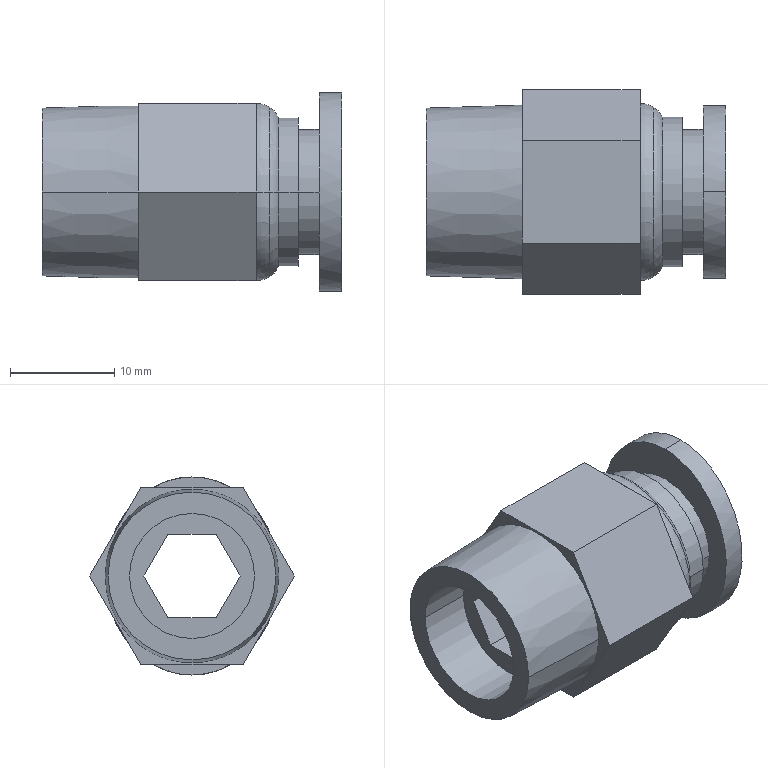Part | Creo | 1 solid | 45 faces | box 28.7 x 19.63 x 19 mm | volume 3914 mm3 | plane 25 | cylinder 8 | torus 8 | cone 2 | other 2 | commonest cylinder face diameters 12 x4 10 x2 14.36 x2
STEP:
#1=CARTESIAN_POINT('',(309.,102.978,120.));
#2=VERTEX_POINT('',#1);
#3=CARTESIAN_POINT('',(309.,114.978,120.));
#4=VERTEX_POINT('',#3);
#5=CARTESIAN_POINT('',(309.,108.978,120.));
#6=DIRECTION('',(-1.,0.,0.));
#7=DIRECTION('',(0.,-1.,0.));
#8=AXIS2_PLACEMENT_3D('',#5,#6,#7);
#9=CIRCLE('',#8,6.);
#10=EDGE_CURVE('',#2,#4,#9,.T.);
#11=ORIENTED_EDGE('',*,*,#10,.F.);
#12=CARTESIAN_POINT('',(309.,108.978,120.));
#13=DIRECTION('',(-1.,0.,0.));
#14=DIRECTION('',(0.,1.,0.));
#15=AXIS2_PLACEMENT_3D('',#12,#13,#14);
#16=CIRCLE('',#15,6.);
#17=EDGE_CURVE('',#4,#2,#16,.T.);
#18=ORIENTED_EDGE('',*,*,#17,.F.);
#19=EDGE_LOOP('',(#11,#18));
#20=FACE_OUTER_BOUND('',#19,.F.);
#21=CARTESIAN_POINT('',(309.,111.287,116.));
#22=VERTEX_POINT('',#21);
#23=CARTESIAN_POINT('',(309.,113.597,120.));
#24=VERTEX_POINT('',#23);
#25=CARTESIAN_POINT('',(309.,111.287,116.));
#26=DIRECTION('',(0.,0.5,0.866));
#27=VECTOR('',#26,4.619);
#28=LINE('',#25,#27);
#29=EDGE_CURVE('',#22,#24,#28,.T.);
#30=ORIENTED_EDGE('',*,*,#29,.F.);
#31=CARTESIAN_POINT('',(309.,106.668,116.));
#32=VERTEX_POINT('',#31);
#33=CARTESIAN_POINT('',(309.,106.668,116.));
#34=DIRECTION('',(0.,1.,0.));
#35=VECTOR('',#34,4.619);
#36=LINE('',#33,#35);
#37=EDGE_CURVE('',#32,#22,#36,.T.);
#38=ORIENTED_EDGE('',*,*,#37,.F.);
#39=CARTESIAN_POINT('',(309.,104.359,120.));
#40=VERTEX_POINT('',#39);
#41=CARTESIAN_POINT('',(309.,104.359,120.));
#42=DIRECTION('',(0.,0.5,-0.866));
#43=VECTOR('',#42,4.619);
#44=LINE('',#41,#43);
#45=EDGE_CURVE('',#40,#32,#44,.T.);
#46=ORIENTED_EDGE('',*,*,#45,.F.);
#47=CARTESIAN_POINT('',(309.,106.668,124.));
#48=VERTEX_POINT('',#47);
#49=CARTESIAN_POINT('',(309.,106.668,124.));
#50=DIRECTION('',(0.,-0.5,-0.866));
#51=VECTOR('',#50,4.619);
#52=LINE('',#49,#51);
#53=EDGE_CURVE('',#48,#40,#52,.T.);
#54=ORIENTED_EDGE('',*,*,#53,.F.);
#55=CARTESIAN_POINT('',(309.,111.287,124.));
#56=VERTEX_POINT('',#55);
#57=CARTESIAN_POINT('',(309.,111.287,124.));
#58=DIRECTION('',(0.,-1.,0.));
#59=VECTOR('',#58,4.619);
#60=LINE('',#57,#59);
#61=EDGE_CURVE('',#56,#48,#60,.T.);
#62=ORIENTED_EDGE('',*,*,#61,.F.);
#63=CARTESIAN_POINT('',(309.,113.597,120.));
#64=DIRECTION('',(0.,-0.5,0.866));
#65=VECTOR('',#64,4.619);
#66=LINE('',#63,#65);
#67=EDGE_CURVE('',#24,#56,#66,.T.);
#68=ORIENTED_EDGE('',*,*,#67,.F.);
#69=EDGE_LOOP('',(#30,#38,#46,#54,#62,#68));
#70=FACE_BOUND('',#69,.F.);
#71=CARTESIAN_POINT('',(309.,108.978,126.));
#72=DIRECTION('',(1.,0.,0.));
#73=DIRECTION('',(0.,1.,0.));
#74=AXIS2_PLACEMENT_3D('',#71,#72,#73);
#75=PLANE('',#74);
#76=ADVANCED_FACE('',(#20,#70),#75,.F.);
#77=CARTESIAN_POINT('',(303.8,114.978,120.));
#78=VERTEX_POINT('',#77);
#79=CARTESIAN_POINT('',(303.8,102.978,120.));
#80=VERTEX_POINT('',#79);
#81=CARTESIAN_POINT('',(303.8,108.978,120.));
#82=DIRECTION('',(1.,0.,0.));
#83=DIRECTION('',(0.,1.,0.));
#84=AXIS2_PLACEMENT_3D('',#81,#82,#83);
#85=CIRCLE('',#84,6.);
#86=EDGE_CURVE('',#78,#80,#85,.T.);
#87=ORIENTED_EDGE('',*,*,#86,.T.);
#88=CARTESIAN_POINT('',(309.,102.978,120.));
#89=DIRECTION('',(-1.,0.,0.));
#90=VECTOR('',#89,5.2);
#91=LINE('',#88,#90);
#92=EDGE_CURVE('',#2,#80,#91,.T.);
#93=ORIENTED_EDGE('',*,*,#92,.F.);
#94=ORIENTED_EDGE('',*,*,#10,.T.);
#95=CARTESIAN_POINT('',(309.,114.978,120.));
#96=DIRECTION('',(-1.,0.,0.));
#97=VECTOR('',#96,5.2);
#98=LINE('',#95,#97);
#99=EDGE_CURVE('',#4,#78,#98,.T.);
#100=ORIENTED_EDGE('',*,*,#99,.T.);
#101=EDGE_LOOP('',(#87,#93,#94,#100));
#102=FACE_OUTER_BOUND('',#101,.F.);
#103=CARTESIAN_POINT('',(335.,108.978,120.));
#104=DIRECTION('',(-1.,0.,0.));
#105=DIRECTION('',(0.,-1.,0.));
#106=AXIS2_PLACEMENT_3D('',#103,#104,#105);
#107=CYLINDRICAL_SURFACE('',#106,6.);
#108=ADVANCED_FACE('',(#102),#107,.F.);
#109=CARTESIAN_POINT('',(303.8,117.023,120.));
#110=VERTEX_POINT('',#109);
#111=CARTESIAN_POINT('',(303.8,100.933,120.));
#112=VERTEX_POINT('',#111);
#113=CARTESIAN_POINT('',(303.8,108.978,120.));
#114=DIRECTION('',(-1.,0.,0.));
#115=DIRECTION('',(0.,1.,0.));
#116=AXIS2_PLACEMENT_3D('',#113,#114,#115);
#117=CIRCLE('',#116,8.045);
#118=EDGE_CURVE('',#110,#112,#117,.T.);
#119=ORIENTED_EDGE('',*,*,#118,.F.);
#120=CARTESIAN_POINT('',(303.8,108.978,120.));
#121=DIRECTION('',(-1.,0.,0.));
#122=DIRECTION('',(0.,-1.,0.));
#123=AXIS2_PLACEMENT_3D('',#120,#121,#122);
#124=CIRCLE('',#123,8.045);
#125=EDGE_CURVE('',#112,#110,#124,.T.);
#126=ORIENTED_EDGE('',*,*,#125,.F.);
#127=EDGE_LOOP('',(#119,#126));
#128=FACE_OUTER_BOUND('',#127,.F.);
#129=CARTESIAN_POINT('',(303.8,108.978,120.));
#130=DIRECTION('',(1.,0.,0.));
#131=DIRECTION('',(0.,-1.,0.));
#132=AXIS2_PLACEMENT_3D('',#129,#130,#131);
#133=CIRCLE('',#132,6.);
#134=EDGE_CURVE('',#80,#78,#133,.T.);
#135=ORIENTED_EDGE('',*,*,#134,.F.);
#136=ORIENTED_EDGE('',*,*,#86,.F.);
#137=EDGE_LOOP('',(#135,#136));
#138=FACE_BOUND('',#137,.F.);
#139=CARTESIAN_POINT('',(303.8,108.978,128.045));
#140=DIRECTION('',(-1.,0.,0.));
#141=DIRECTION('',(0.,-1.,0.));
#142=AXIS2_PLACEMENT_3D('',#139,#140,#141);
#143=PLANE('',#142);
#144=ADVANCED_FACE('',(#128,#138),#143,.T.);
#145=ORIENTED_EDGE('',*,*,#134,.T.);
#146=ORIENTED_EDGE('',*,*,#99,.F.);
#147=ORIENTED_EDGE('',*,*,#17,.T.);
#148=ORIENTED_EDGE('',*,*,#92,.T.);
#149=EDGE_LOOP('',(#145,#146,#147,#148));
#150=FACE_OUTER_BOUND('',#149,.F.);
#151=CARTESIAN_POINT('',(335.,108.978,120.));
#152=DIRECTION('',(-1.,0.,0.));
#153=DIRECTION('',(0.,-1.,0.));
#154=AXIS2_PLACEMENT_3D('',#151,#152,#153);
#155=CYLINDRICAL_SURFACE('',#154,6.);
#156=ADVANCED_FACE('',(#150),#155,.F.);
#157=ORIENTED_EDGE('',*,*,#118,.T.);
#158=CARTESIAN_POINT('',(313.,100.648,120.));
#159=VERTEX_POINT('',#158);
#160=CARTESIAN_POINT('',(303.8,100.933,120.));
#161=DIRECTION('',(0.9995,-0.03097,0.));
#162=VECTOR('',#161,9.204);
#163=LINE('',#160,#162);
#164=EDGE_CURVE('',#112,#159,#163,.T.);
#165=ORIENTED_EDGE('',*,*,#164,.T.);
#166=CARTESIAN_POINT('',(313.,117.308,120.));
#167=VERTEX_POINT('',#166);
#168=CARTESIAN_POINT('',(313.,108.978,120.));
#169=DIRECTION('',(1.,0.,0.));
#170=DIRECTION('',(0.,-1.,0.));
#171=AXIS2_PLACEMENT_3D('',#168,#169,#170);
#172=CIRCLE('',#171,8.33);
#173=EDGE_CURVE('',#159,#167,#172,.T.);
#174=ORIENTED_EDGE('',*,*,#173,.T.);
#175=CARTESIAN_POINT('',(303.8,117.023,120.));
#176=DIRECTION('',(0.9995,0.03097,0.));
#177=VECTOR('',#176,9.204);
#178=LINE('',#175,#177);
#179=EDGE_CURVE('',#110,#167,#178,.T.);
#180=ORIENTED_EDGE('',*,*,#179,.F.);
#181=EDGE_LOOP('',(#157,#165,#174,#180));
#182=FACE_OUTER_BOUND('',#181,.F.);
#183=CARTESIAN_POINT('',(308.4,108.978,120.));
#184=DIRECTION('',(1.,0.,0.));
#185=DIRECTION('',(0.,1.,0.));
#186=AXIS2_PLACEMENT_3D('',#183,#184,#185);
#187=CONICAL_SURFACE('',#186,8.187,1.775);
#188=ADVANCED_FACE('',(#182),#187,.T.);
#189=ORIENTED_EDGE('',*,*,#125,.T.);
#190=ORIENTED_EDGE('',*,*,#179,.T.);
#191=CARTESIAN_POINT('',(313.,108.978,120.));
#192=DIRECTION('',(1.,0.,0.));
#193=DIRECTION('',(0.,1.,0.));
#194=AXIS2_PLACEMENT_3D('',#191,#192,#193);
#195=CIRCLE('',#194,8.33);
#196=EDGE_CURVE('',#167,#159,#195,.T.);
#197=ORIENTED_EDGE('',*,*,#196,.T.);
#198=ORIENTED_EDGE('',*,*,#164,.F.);
#199=EDGE_LOOP('',(#189,#190,#197,#198));
#200=FACE_OUTER_BOUND('',#199,.F.);
#201=CARTESIAN_POINT('',(308.4,108.978,120.));
#202=DIRECTION('',(1.,0.,0.));
#203=DIRECTION('',(0.,1.,0.));
#204=AXIS2_PLACEMENT_3D('',#201,#202,#203);
#205=CONICAL_SURFACE('',#204,8.187,1.775);
#206=ADVANCED_FACE('',(#200),#205,.T.);
#207=CARTESIAN_POINT('',(313.,99.163,120.));
#208=VERTEX_POINT('',#207);
#209=CARTESIAN_POINT('',(313.,104.07,128.5));
#210=VERTEX_POINT('',#209);
#211=CARTESIAN_POINT('',(313.,99.163,120.));
#212=DIRECTION('',(0.,0.5,0.866));
#213=VECTOR('',#212,9.815);
#214=LINE('',#211,#213);
#215=EDGE_CURVE('',#208,#210,#214,.T.);
#216=ORIENTED_EDGE('',*,*,#215,.F.);
#217=CARTESIAN_POINT('',(313.,104.07,111.5));
#218=VERTEX_POINT('',#217);
#219=CARTESIAN_POINT('',(313.,104.07,111.5));
#220=DIRECTION('',(0.,-0.5,0.866));
#221=VECTOR('',#220,9.815);
#222=LINE('',#219,#221);
#223=EDGE_CURVE('',#218,#208,#222,.T.);
#224=ORIENTED_EDGE('',*,*,#223,.F.);
#225=CARTESIAN_POINT('',(313.,113.885,111.5));
#226=VERTEX_POINT('',#225);
#227=CARTESIAN_POINT('',(313.,104.07,111.5));
#228=DIRECTION('',(0.,1.,0.));
#229=VECTOR('',#228,9.815);
#230=LINE('',#227,#229);
#231=EDGE_CURVE('',#218,#226,#230,.T.);
#232=ORIENTED_EDGE('',*,*,#231,.T.);
#233=CARTESIAN_POINT('',(313.,118.793,120.));
#234=VERTEX_POINT('',#233);
#235=CARTESIAN_POINT('',(313.,118.793,120.));
#236=DIRECTION('',(0.,-0.5,-0.866));
#237=VECTOR('',#236,9.815);
#238=LINE('',#235,#237);
#239=EDGE_CURVE('',#234,#226,#238,.T.);
#240=ORIENTED_EDGE('',*,*,#239,.F.);
#241=CARTESIAN_POINT('',(313.,113.885,128.5));
#242=VERTEX_POINT('',#241);
#243=CARTESIAN_POINT('',(313.,113.885,128.5));
#244=DIRECTION('',(0.,0.5,-0.866));
#245=VECTOR('',#244,9.815);
#246=LINE('',#243,#245);
#247=EDGE_CURVE('',#242,#234,#246,.T.);
#248=ORIENTED_EDGE('',*,*,#247,.F.);
#249=CARTESIAN_POINT('',(313.,113.885,128.5));
#250=DIRECTION('',(0.,-1.,0.));
#251=VECTOR('',#250,9.815);
#252=LINE('',#249,#251);
#253=EDGE_CURVE('',#242,#210,#252,.T.);
#254=ORIENTED_EDGE('',*,*,#253,.T.);
#255=EDGE_LOOP('',(#216,#224,#232,#240,#248,#254));
#256=FACE_OUTER_BOUND('',#255,.F.);
#257=ORIENTED_EDGE('',*,*,#196,.F.);
#258=ORIENTED_EDGE('',*,*,#173,.F.);
#259=EDGE_LOOP('',(#257,#258));
#260=FACE_BOUND('',#259,.F.);
#261=CARTESIAN_POINT('',(313.,108.978,128.4));
#262=DIRECTION('',(-1.,0.,0.));
#263=DIRECTION('',(0.,-1.,0.));
#264=AXIS2_PLACEMENT_3D('',#261,#262,#263);
#265=PLANE('',#264);
#266=ADVANCED_FACE('',(#256,#260),#265,.T.);
#267=ORIENTED_EDGE('',*,*,#215,.T.);
#268=CARTESIAN_POINT('',(324.3,104.07,128.5));
#269=VERTEX_POINT('',#268);
#270=CARTESIAN_POINT('',(313.,104.07,128.5));
#271=DIRECTION('',(1.,0.,0.));
#272=VECTOR('',#271,11.3);
#273=LINE('',#270,#272);
#274=EDGE_CURVE('',#210,#269,#273,.T.);
#275=ORIENTED_EDGE('',*,*,#274,.T.);
#276=CARTESIAN_POINT('',(324.3,101.617,124.25));
#277=VERTEX_POINT('',#276);
#278=CARTESIAN_POINT('',(324.3,104.07,128.5));
#279=DIRECTION('',(0.,-0.5,-0.866));
#280=VECTOR('',#279,4.907);
#281=LINE('',#278,#280);
#282=EDGE_CURVE('',#269,#277,#281,.T.);
#283=ORIENTED_EDGE('',*,*,#282,.T.);
#284=CARTESIAN_POINT('',(324.3,99.163,120.));
#285=VERTEX_POINT('',#284);
#286=CARTESIAN_POINT('',(324.3,101.617,124.25));
#287=DIRECTION('',(0.,-0.5,-0.866));
#288=VECTOR('',#287,4.907);
#289=LINE('',#286,#288);
#290=EDGE_CURVE('',#277,#285,#289,.T.);
#291=ORIENTED_EDGE('',*,*,#290,.T.);
#292=CARTESIAN_POINT('',(313.,99.163,120.));
#293=DIRECTION('',(1.,0.,0.));
#294=VECTOR('',#293,11.3);
#295=LINE('',#292,#294);
#296=EDGE_CURVE('',#208,#285,#295,.T.);
#297=ORIENTED_EDGE('',*,*,#296,.F.);
#298=EDGE_LOOP('',(#267,#275,#283,#291,#297));
#299=FACE_OUTER_BOUND('',#298,.F.);
#300=CARTESIAN_POINT('',(324.3,99.163,120.));
#301=DIRECTION('',(0.,-0.866,0.5));
#302=DIRECTION('',(0.,-0.5,-0.866));
#303=AXIS2_PLACEMENT_3D('',#300,#301,#302);
#304=PLANE('',#303);
#305=ADVANCED_FACE('',(#299),#304,.T.);
#306=ORIENTED_EDGE('',*,*,#253,.F.);
#307=CARTESIAN_POINT('',(324.3,113.885,128.5));
#308=VERTEX_POINT('',#307);
#309=CARTESIAN_POINT('',(313.,113.885,128.5));
#310=DIRECTION('',(1.,0.,0.));
#311=VECTOR('',#310,11.3);
#312=LINE('',#309,#311);
#313=EDGE_CURVE('',#242,#308,#312,.T.);
#314=ORIENTED_EDGE('',*,*,#313,.T.);
#315=CARTESIAN_POINT('',(324.3,108.978,128.5));
#316=VERTEX_POINT('',#315);
#317=CARTESIAN_POINT('',(324.3,113.885,128.5));
#318=DIRECTION('',(0.,-1.,0.));
#319=VECTOR('',#318,4.907);
#320=LINE('',#317,#319);
#321=EDGE_CURVE('',#308,#316,#320,.T.);
#322=ORIENTED_EDGE('',*,*,#321,.T.);
#323=CARTESIAN_POINT('',(324.3,108.978,128.5));
#324=DIRECTION('',(0.,-1.,0.));
#325=VECTOR('',#324,4.907);
#326=LINE('',#323,#325);
#327=EDGE_CURVE('',#316,#269,#326,.T.);
#328=ORIENTED_EDGE('',*,*,#327,.T.);
#329=ORIENTED_EDGE('',*,*,#274,.F.);
#330=EDGE_LOOP('',(#306,#314,#322,#328,#329));
#331=FACE_OUTER_BOUND('',#330,.F.);
#332=CARTESIAN_POINT('',(324.3,104.07,128.5));
#333=DIRECTION('',(0.,0.,1.));
#334=DIRECTION('',(1.,0.,0.));
#335=AXIS2_PLACEMENT_3D('',#332,#333,#334);
#336=PLANE('',#335);
#337=ADVANCED_FACE('',(#331),#336,.T.);
#338=CARTESIAN_POINT('',(324.3,118.793,120.));
#339=VERTEX_POINT('',#338);
#340=CARTESIAN_POINT('',(313.,118.793,120.));
#341=DIRECTION('',(1.,0.,0.));
#342=VECTOR('',#341,11.3);
#343=LINE('',#340,#342);
#344=EDGE_CURVE('',#234,#339,#343,.T.);
#345=ORIENTED_EDGE('',*,*,#344,.T.);
#346=CARTESIAN_POINT('',(324.3,116.339,124.25));
#347=VERTEX_POINT('',#346);
#348=CARTESIAN_POINT('',(324.3,118.793,120.));
#349=DIRECTION('',(0.,-0.5,0.866));
#350=VECTOR('',#349,4.907);
#351=LINE('',#348,#350);
#352=EDGE_CURVE('',#339,#347,#351,.T.);
#353=ORIENTED_EDGE('',*,*,#352,.T.);
#354=CARTESIAN_POINT('',(324.3,116.339,124.25));
#355=DIRECTION('',(0.,-0.5,0.866));
#356=VECTOR('',#355,4.907);
#357=LINE('',#354,#356);
#358=EDGE_CURVE('',#347,#308,#357,.T.);
#359=ORIENTED_EDGE('',*,*,#358,.T.);
#360=ORIENTED_EDGE('',*,*,#313,.F.);
#361=ORIENTED_EDGE('',*,*,#247,.T.);
#362=EDGE_LOOP('',(#345,#353,#359,#360,#361));
#363=FACE_OUTER_BOUND('',#362,.F.);
#364=CARTESIAN_POINT('',(324.3,113.885,128.5));
#365=DIRECTION('',(0.,0.866,0.5));
#366=DIRECTION('',(0.,-0.5,0.866));
#367=AXIS2_PLACEMENT_3D('',#364,#365,#366);
#368=PLANE('',#367);
#369=ADVANCED_FACE('',(#363),#368,.T.);
#370=ORIENTED_EDGE('',*,*,#239,.T.);
#371=CARTESIAN_POINT('',(324.3,113.885,111.5));
#372=VERTEX_POINT('',#371);
#373=CARTESIAN_POINT('',(313.,113.885,111.5));
#374=DIRECTION('',(1.,0.,0.));
#375=VECTOR('',#374,11.3);
#376=LINE('',#373,#375);
#377=EDGE_CURVE('',#226,#372,#376,.T.);
#378=ORIENTED_EDGE('',*,*,#377,.T.);
#379=CARTESIAN_POINT('',(324.3,116.339,115.75));
#380=VERTEX_POINT('',#379);
#381=CARTESIAN_POINT('',(324.3,113.885,111.5));
#382=DIRECTION('',(0.,0.5,0.866));
#383=VECTOR('',#382,4.907);
#384=LINE('',#381,#383);
#385=EDGE_CURVE('',#372,#380,#384,.T.);
#386=ORIENTED_EDGE('',*,*,#385,.T.);
#387=CARTESIAN_POINT('',(324.3,116.339,115.75));
#388=DIRECTION('',(0.,0.5,0.866));
#389=VECTOR('',#388,4.907);
#390=LINE('',#387,#389);
#391=EDGE_CURVE('',#380,#339,#390,.T.);
#392=ORIENTED_EDGE('',*,*,#391,.T.);
#393=ORIENTED_EDGE('',*,*,#344,.F.);
#394=EDGE_LOOP('',(#370,#378,#386,#392,#393));
#395=FACE_OUTER_BOUND('',#394,.F.);
#396=CARTESIAN_POINT('',(324.3,118.793,120.));
#397=DIRECTION('',(0.,0.866,-0.5));
#398=DIRECTION('',(0.,0.5,0.866));
#399=AXIS2_PLACEMENT_3D('',#396,#397,#398);
#400=PLANE('',#399);
#401=ADVANCED_FACE('',(#395),#400,.T.);
#402=ORIENTED_EDGE('',*,*,#231,.F.);
#403=CARTESIAN_POINT('',(324.3,104.07,111.5));
#404=VERTEX_POINT('',#403);
#405=CARTESIAN_POINT('',(313.,104.07,111.5));
#406=DIRECTION('',(1.,0.,0.));
#407=VECTOR('',#406,11.3);
#408=LINE('',#405,#407);
#409=EDGE_CURVE('',#218,#404,#408,.T.);
#410=ORIENTED_EDGE('',*,*,#409,.T.);
#411=CARTESIAN_POINT('',(324.3,108.978,111.5));
#412=VERTEX_POINT('',#411);
#413=CARTESIAN_POINT('',(324.3,104.07,111.5));
#414=DIRECTION('',(0.,1.,0.));
#415=VECTOR('',#414,4.907);
#416=LINE('',#413,#415);
#417=EDGE_CURVE('',#404,#412,#416,.T.);
#418=ORIENTED_EDGE('',*,*,#417,.T.);
#419=CARTESIAN_POINT('',(324.3,108.978,111.5));
#420=DIRECTION('',(0.,1.,0.));
#421=VECTOR('',#420,4.907);
#422=LINE('',#419,#421);
#423=EDGE_CURVE('',#412,#372,#422,.T.);
#424=ORIENTED_EDGE('',*,*,#423,.T.);
#425=ORIENTED_EDGE('',*,*,#377,.F.);
#426=EDGE_LOOP('',(#402,#410,#418,#424,#425));
#427=FACE_OUTER_BOUND('',#426,.F.);
#428=CARTESIAN_POINT('',(324.3,113.885,111.5));
#429=DIRECTION('',(0.,0.,-1.));
#430=DIRECTION('',(0.,1.,0.));
#431=AXIS2_PLACEMENT_3D('',#428,#429,#430);
#432=PLANE('',#431);
#433=ADVANCED_FACE('',(#427),#432,.T.);
#434=ORIENTED_EDGE('',*,*,#223,.T.);
#435=ORIENTED_EDGE('',*,*,#296,.T.);
#436=CARTESIAN_POINT('',(324.3,101.617,115.75));
#437=VERTEX_POINT('',#436);
#438=CARTESIAN_POINT('',(324.3,99.163,120.));
#439=DIRECTION('',(0.,0.5,-0.866));
#440=VECTOR('',#439,4.907);
#441=LINE('',#438,#440);
#442=EDGE_CURVE('',#285,#437,#441,.T.);
#443=ORIENTED_EDGE('',*,*,#442,.T.);
#444=CARTESIAN_POINT('',(324.3,101.617,115.75));
#445=DIRECTION('',(0.,0.5,-0.866));
#446=VECTOR('',#445,4.907);
#447=LINE('',#444,#446);
#448=EDGE_CURVE('',#437,#404,#447,.T.);
#449=ORIENTED_EDGE('',*,*,#448,.T.);
#450=ORIENTED_EDGE('',*,*,#409,.F.);
#451=EDGE_LOOP('',(#434,#435,#443,#449,#450));
#452=FACE_OUTER_BOUND('',#451,.F.);
#453=CARTESIAN_POINT('',(324.3,104.07,111.5));
#454=DIRECTION('',(0.,-0.866,-0.5));
#455=DIRECTION('',(0.,0.5,-0.866));
#456=AXIS2_PLACEMENT_3D('',#453,#454,#455);
#457=PLANE('',#456);
#458=ADVANCED_FACE('',(#452),#457,.T.);
#459=CARTESIAN_POINT('',(324.3,100.478,120.));
#460=VERTEX_POINT('',#459);
#461=CARTESIAN_POINT('',(324.3,108.978,120.));
#462=DIRECTION('',(-1.,0.,0.));
#463=DIRECTION('',(0.,-0.866,-0.5));
#464=AXIS2_PLACEMENT_3D('',#461,#462,#463);
#465=CIRCLE('',#464,8.5);
#466=EDGE_CURVE('',#437,#460,#465,.T.);
#467=ORIENTED_EDGE('',*,*,#466,.F.);
#468=ORIENTED_EDGE('',*,*,#442,.F.);
#469=ORIENTED_EDGE('',*,*,#290,.F.);
#470=CARTESIAN_POINT('',(324.3,108.978,120.));
#471=DIRECTION('',(-1.,0.,0.));
#472=DIRECTION('',(0.,-1.,0.));
#473=AXIS2_PLACEMENT_3D('',#470,#471,#472);
#474=CIRCLE('',#473,8.5);
#475=EDGE_CURVE('',#460,#277,#474,.T.);
#476=ORIENTED_EDGE('',*,*,#475,.F.);
#477=EDGE_LOOP('',(#467,#468,#469,#476));
#478=FACE_OUTER_BOUND('',#477,.F.);
#479=CARTESIAN_POINT('',(324.3,108.978,120.));
#480=DIRECTION('',(-1.,0.,0.));
#481=DIRECTION('',(0.,-1.,0.));
#482=AXIS2_PLACEMENT_3D('',#479,#480,#481);
#483=PLANE('',#482);
#484=ADVANCED_FACE('',(#478),#483,.F.);
#485=ORIENTED_EDGE('',*,*,#466,.T.);
#486=CARTESIAN_POINT('',(325.561,100.834,120.));
#487=VERTEX_POINT('',#486);
#488=CARTESIAN_POINT('',(324.3,102.889,120.));
#489=DIRECTION('',(0.,0.,1.));
#490=DIRECTION('',(0.,-1.,0.));
#491=AXIS2_PLACEMENT_3D('',#488,#489,#490);
#492=CIRCLE('',#491,2.411);
#493=EDGE_CURVE('',#460,#487,#492,.T.);
#494=ORIENTED_EDGE('',*,*,#493,.T.);
#495=CARTESIAN_POINT('',(325.561,117.121,120.));
#496=VERTEX_POINT('',#495);
#497=CARTESIAN_POINT('',(325.561,108.978,120.));
#498=DIRECTION('',(1.,0.,0.));
#499=DIRECTION('',(0.,-1.,0.));
#500=AXIS2_PLACEMENT_3D('',#497,#498,#499);
#501=CIRCLE('',#500,8.144);
#502=EDGE_CURVE('',#487,#496,#501,.T.);
#503=ORIENTED_EDGE('',*,*,#502,.T.);
#504=CARTESIAN_POINT('',(324.3,117.478,120.));
#505=VERTEX_POINT('',#504);
#506=CARTESIAN_POINT('',(324.3,115.067,120.));
#507=DIRECTION('',(0.,0.,-1.));
#508=DIRECTION('',(0.,1.,0.));
#509=AXIS2_PLACEMENT_3D('',#506,#507,#508);
#510=CIRCLE('',#509,2.411);
#511=EDGE_CURVE('',#505,#496,#510,.T.);
#512=ORIENTED_EDGE('',*,*,#511,.F.);
#513=CARTESIAN_POINT('',(324.3,108.978,120.));
#514=DIRECTION('',(-1.,0.,0.));
#515=DIRECTION('',(0.,1.,0.));
#516=AXIS2_PLACEMENT_3D('',#513,#514,#515);
#517=CIRCLE('',#516,8.5);
#518=EDGE_CURVE('',#505,#380,#517,.T.);
#519=ORIENTED_EDGE('',*,*,#518,.T.);
#520=CARTESIAN_POINT('',(324.3,108.978,120.));
#521=DIRECTION('',(-1.,0.,0.));
#522=DIRECTION('',(0.,0.866,-0.5));
#523=AXIS2_PLACEMENT_3D('',#520,#521,#522);
#524=CIRCLE('',#523,8.5);
#525=EDGE_CURVE('',#380,#412,#524,.T.);
#526=ORIENTED_EDGE('',*,*,#525,.T.);
#527=CARTESIAN_POINT('',(324.3,108.978,120.));
#528=DIRECTION('',(-1.,0.,0.));
#529=DIRECTION('',(0.,0.,-1.));
#530=AXIS2_PLACEMENT_3D('',#527,#528,#529);
#531=CIRCLE('',#530,8.5);
#532=EDGE_CURVE('',#412,#437,#531,.T.);
#533=ORIENTED_EDGE('',*,*,#532,.T.);
#534=EDGE_LOOP('',(#485,#494,#503,#512,#519,#526,#533));
#535=FACE_OUTER_BOUND('',#534,.F.);
#536=CARTESIAN_POINT('',(324.3,108.978,120.));
#537=DIRECTION('',(1.,0.,0.));
#538=DIRECTION('',(0.,1.,0.));
#539=AXIS2_PLACEMENT_3D('',#536,#537,#538);
#540=TOROIDAL_SURFACE('',#539,6.089,2.411);
#541=ADVANCED_FACE('',(#535),#540,.T.);
#542=CARTESIAN_POINT('',(324.3,108.978,120.));
#543=DIRECTION('',(-1.,0.,0.));
#544=DIRECTION('',(0.,0.,1.));
#545=AXIS2_PLACEMENT_3D('',#542,#543,#544);
#546=CIRCLE('',#545,8.5);
#547=EDGE_CURVE('',#316,#347,#546,.T.);
#548=ORIENTED_EDGE('',*,*,#547,.T.);
#549=CARTESIAN_POINT('',(324.3,108.978,120.));
#550=DIRECTION('',(-1.,0.,0.));
#551=DIRECTION('',(0.,0.866,0.5));
#552=AXIS2_PLACEMENT_3D('',#549,#550,#551);
#553=CIRCLE('',#552,8.5);
#554=EDGE_CURVE('',#347,#505,#553,.T.);
#555=ORIENTED_EDGE('',*,*,#554,.T.);
#556=ORIENTED_EDGE('',*,*,#511,.T.);
#557=CARTESIAN_POINT('',(325.561,108.978,120.));
#558=DIRECTION('',(1.,0.,0.));
#559=DIRECTION('',(0.,1.,0.));
#560=AXIS2_PLACEMENT_3D('',#557,#558,#559);
#561=CIRCLE('',#560,8.144);
#562=EDGE_CURVE('',#496,#487,#561,.T.);
#563=ORIENTED_EDGE('',*,*,#562,.T.);
#564=ORIENTED_EDGE('',*,*,#493,.F.);
#565=ORIENTED_EDGE('',*,*,#475,.T.);
#566=CARTESIAN_POINT('',(324.3,108.978,120.));
#567=DIRECTION('',(-1.,0.,0.));
#568=DIRECTION('',(0.,-0.866,0.5));
#569=AXIS2_PLACEMENT_3D('',#566,#567,#568);
#570=CIRCLE('',#569,8.5);
#571=EDGE_CURVE('',#277,#316,#570,.T.);
#572=ORIENTED_EDGE('',*,*,#571,.T.);
#573=EDGE_LOOP('',(#548,#555,#556,#563,#564,#565,#572));
#574=FACE_OUTER_BOUND('',#573,.F.);
#575=CARTESIAN_POINT('',(324.3,108.978,120.));
#576=DIRECTION('',(1.,0.,0.));
#577=DIRECTION('',(0.,1.,0.));
#578=AXIS2_PLACEMENT_3D('',#575,#576,#577);
#579=TOROIDAL_SURFACE('',#578,6.089,2.411);
#580=ADVANCED_FACE('',(#574),#579,.T.);
#581=ORIENTED_EDGE('',*,*,#547,.F.);
#582=ORIENTED_EDGE('',*,*,#321,.F.);
#583=ORIENTED_EDGE('',*,*,#358,.F.);
#584=EDGE_LOOP('',(#581,#582,#583));
#585=FACE_OUTER_BOUND('',#584,.F.);
#586=CARTESIAN_POINT('',(324.3,108.978,120.));
#587=DIRECTION('',(-1.,0.,0.));
#588=DIRECTION('',(0.,-1.,0.));
#589=AXIS2_PLACEMENT_3D('',#586,#587,#588);
#590=PLANE('',#589);
#591=ADVANCED_FACE('',(#585),#590,.F.);
#592=ORIENTED_EDGE('',*,*,#518,.F.);
#593=ORIENTED_EDGE('',*,*,#554,.F.);
#594=ORIENTED_EDGE('',*,*,#352,.F.);
#595=ORIENTED_EDGE('',*,*,#391,.F.);
#596=EDGE_LOOP('',(#592,#593,#594,#595));
#597=FACE_OUTER_BOUND('',#596,.F.);
#598=CARTESIAN_POINT('',(324.3,108.978,120.));
#599=DIRECTION('',(-1.,0.,0.));
#600=DIRECTION('',(0.,-1.,0.));
#601=AXIS2_PLACEMENT_3D('',#598,#599,#600);
#602=PLANE('',#601);
#603=ADVANCED_FACE('',(#597),#602,.F.);
#604=CARTESIAN_POINT('',(326.45,101.798,120.));
#605=VERTEX_POINT('',#604);
#606=CARTESIAN_POINT('',(326.45,116.158,120.));
#607=VERTEX_POINT('',#606);
#608=CARTESIAN_POINT('',(326.45,108.978,120.));
#609=DIRECTION('',(-1.,0.,0.));
#610=DIRECTION('',(0.,-1.,0.));
#611=AXIS2_PLACEMENT_3D('',#608,#609,#610);
#612=CIRCLE('',#611,7.18);
#613=EDGE_CURVE('',#605,#607,#612,.T.);
#614=ORIENTED_EDGE('',*,*,#613,.F.);
#615=CARTESIAN_POINT('',(324.3,102.889,120.));
#616=DIRECTION('',(0.,0.,1.));
#617=DIRECTION('',(0.5232,-0.8522,0.));
#618=AXIS2_PLACEMENT_3D('',#615,#616,#617);
#619=CIRCLE('',#618,2.411);
#620=EDGE_CURVE('',#487,#605,#619,.T.);
#621=ORIENTED_EDGE('',*,*,#620,.F.);
#622=ORIENTED_EDGE('',*,*,#562,.F.);
#623=CARTESIAN_POINT('',(324.3,115.067,120.));
#624=DIRECTION('',(0.,0.,-1.));
#625=DIRECTION('',(0.5232,0.8522,0.));
#626=AXIS2_PLACEMENT_3D('',#623,#624,#625);
#627=CIRCLE('',#626,2.411);
#628=EDGE_CURVE('',#496,#607,#627,.T.);
#629=ORIENTED_EDGE('',*,*,#628,.T.);
#630=EDGE_LOOP('',(#614,#621,#622,#629));
#631=FACE_OUTER_BOUND('',#630,.F.);
#632=CARTESIAN_POINT('',(324.3,108.978,120.));
#633=DIRECTION('',(1.,0.,0.));
#634=DIRECTION('',(0.,1.,0.));
#635=AXIS2_PLACEMENT_3D('',#632,#633,#634);
#636=TOROIDAL_SURFACE('',#635,6.089,2.411);
#637=ADVANCED_FACE('',(#631),#636,.T.);
#638=ORIENTED_EDGE('',*,*,#613,.T.);
#639=CARTESIAN_POINT('',(328.35,116.158,120.));
#640=VERTEX_POINT('',#639);
#641=CARTESIAN_POINT('',(326.45,116.158,120.));
#642=DIRECTION('',(1.,0.,0.));
#643=VECTOR('',#642,1.9);
#644=LINE('',#641,#643);
#645=EDGE_CURVE('',#607,#640,#644,.T.);
#646=ORIENTED_EDGE('',*,*,#645,.T.);
#647=CARTESIAN_POINT('',(328.35,101.798,120.));
#648=VERTEX_POINT('',#647);
#649=CARTESIAN_POINT('',(328.35,108.978,120.));
#650=DIRECTION('',(1.,0.,0.));
#651=DIRECTION('',(0.,1.,0.));
#652=AXIS2_PLACEMENT_3D('',#649,#650,#651);
#653=CIRCLE('',#652,7.18);
#654=EDGE_CURVE('',#640,#648,#653,.T.);
#655=ORIENTED_EDGE('',*,*,#654,.T.);
#656=CARTESIAN_POINT('',(326.45,101.798,120.));
#657=DIRECTION('',(1.,0.,0.));
#658=VECTOR('',#657,1.9);
#659=LINE('',#656,#658);
#660=EDGE_CURVE('',#605,#648,#659,.T.);
#661=ORIENTED_EDGE('',*,*,#660,.F.);
#662=EDGE_LOOP('',(#638,#646,#655,#661));
#663=FACE_OUTER_BOUND('',#662,.F.);
#664=CARTESIAN_POINT('',(335.,108.978,120.));
#665=DIRECTION('',(1.,0.,0.));
#666=DIRECTION('',(0.,1.,0.));
#667=AXIS2_PLACEMENT_3D('',#664,#665,#666);
#668=CYLINDRICAL_SURFACE('',#667,7.18);
#669=ADVANCED_FACE('',(#663),#668,.T.);
#670=CARTESIAN_POINT('',(326.45,108.978,120.));
#671=DIRECTION('',(-1.,0.,0.));
#672=DIRECTION('',(0.,1.,0.));
#673=AXIS2_PLACEMENT_3D('',#670,#671,#672);
#674=CIRCLE('',#673,7.18);
#675=EDGE_CURVE('',#607,#605,#674,.T.);
#676=ORIENTED_EDGE('',*,*,#675,.T.);
#677=ORIENTED_EDGE('',*,*,#660,.T.);
#678=CARTESIAN_POINT('',(328.35,108.978,120.));
#679=DIRECTION('',(1.,0.,0.));
#680=DIRECTION('',(0.,-1.,0.));
#681=AXIS2_PLACEMENT_3D('',#678,#679,#680);
#682=CIRCLE('',#681,7.18);
#683=EDGE_CURVE('',#648,#640,#682,.T.);
#684=ORIENTED_EDGE('',*,*,#683,.T.);
#685=ORIENTED_EDGE('',*,*,#645,.F.);
#686=EDGE_LOOP('',(#676,#677,#684,#685));
#687=FACE_OUTER_BOUND('',#686,.F.);
#688=CARTESIAN_POINT('',(335.,108.978,120.));
#689=DIRECTION('',(1.,0.,0.));
#690=DIRECTION('',(0.,1.,0.));
#691=AXIS2_PLACEMENT_3D('',#688,#689,#690);
#692=CYLINDRICAL_SURFACE('',#691,7.18);
#693=ADVANCED_FACE('',(#687),#692,.T.);
#694=ORIENTED_EDGE('',*,*,#675,.F.);
#695=ORIENTED_EDGE('',*,*,#628,.F.);
#696=ORIENTED_EDGE('',*,*,#502,.F.);
#697=ORIENTED_EDGE('',*,*,#620,.T.);
#698=EDGE_LOOP('',(#694,#695,#696,#697));
#699=FACE_OUTER_BOUND('',#698,.F.);
#700=CARTESIAN_POINT('',(324.3,108.978,120.));
#701=DIRECTION('',(1.,0.,0.));
#702=DIRECTION('',(0.,1.,0.));
#703=AXIS2_PLACEMENT_3D('',#700,#701,#702);
#704=TOROIDAL_SURFACE('',#703,6.089,2.411);
#705=ADVANCED_FACE('',(#699),#704,.T.);
#706=ORIENTED_EDGE('',*,*,#654,.F.);
#707=ORIENTED_EDGE('',*,*,#683,.F.);
#708=EDGE_LOOP('',(#706,#707));
#709=FACE_OUTER_BOUND('',#708,.F.);
#710=CARTESIAN_POINT('',(328.35,114.978,120.));
#711=VERTEX_POINT('',#710);
#712=CARTESIAN_POINT('',(328.35,102.978,120.));
#713=VERTEX_POINT('',#712);
#714=CARTESIAN_POINT('',(328.35,108.978,120.));
#715=DIRECTION('',(-1.,0.,0.));
#716=DIRECTION('',(0.,1.,0.));
#717=AXIS2_PLACEMENT_3D('',#714,#715,#716);
#718=CIRCLE('',#717,6.);
#719=EDGE_CURVE('',#711,#713,#718,.T.);
#720=ORIENTED_EDGE('',*,*,#719,.F.);
#721=CARTESIAN_POINT('',(328.35,108.978,120.));
#722=DIRECTION('',(-1.,0.,0.));
#723=DIRECTION('',(0.,-1.,0.));
#724=AXIS2_PLACEMENT_3D('',#721,#722,#723);
#725=CIRCLE('',#724,6.);
#726=EDGE_CURVE('',#713,#711,#725,.T.);
#727=ORIENTED_EDGE('',*,*,#726,.F.);
#728=EDGE_LOOP('',(#720,#727));
#729=FACE_BOUND('',#728,.F.);
#730=CARTESIAN_POINT('',(328.35,108.978,126.));
#731=DIRECTION('',(1.,0.,0.));
#732=DIRECTION('',(0.,1.,0.));
#733=AXIS2_PLACEMENT_3D('',#730,#731,#732);
#734=PLANE('',#733);
#735=ADVANCED_FACE('',(#709,#729),#734,.T.);
#736=ORIENTED_EDGE('',*,*,#719,.T.);
#737=CARTESIAN_POINT('',(330.35,102.978,120.));
#738=VERTEX_POINT('',#737);
#739=CARTESIAN_POINT('',(328.35,102.978,120.));
#740=DIRECTION('',(1.,0.,0.));
#741=VECTOR('',#740,2.);
#742=LINE('',#739,#741);
#743=EDGE_CURVE('',#713,#738,#742,.T.);
#744=ORIENTED_EDGE('',*,*,#743,.T.);
#745=CARTESIAN_POINT('',(330.35,114.978,120.));
#746=VERTEX_POINT('',#745);
#747=CARTESIAN_POINT('',(330.35,108.978,120.));
#748=DIRECTION('',(1.,0.,0.));
#749=DIRECTION('',(0.,-1.,0.));
#750=AXIS2_PLACEMENT_3D('',#747,#748,#749);
#751=CIRCLE('',#750,6.);
#752=EDGE_CURVE('',#738,#746,#751,.T.);
#753=ORIENTED_EDGE('',*,*,#752,.T.);
#754=CARTESIAN_POINT('',(328.35,114.978,120.));
#755=DIRECTION('',(1.,0.,0.));
#756=VECTOR('',#755,2.);
#757=LINE('',#754,#756);
#758=EDGE_CURVE('',#711,#746,#757,.T.);
#759=ORIENTED_EDGE('',*,*,#758,.F.);
#760=EDGE_LOOP('',(#736,#744,#753,#759));
#761=FACE_OUTER_BOUND('',#760,.F.);
#762=CARTESIAN_POINT('',(335.,108.978,120.));
#763=DIRECTION('',(1.,0.,0.));
#764=DIRECTION('',(0.,1.,0.));
#765=AXIS2_PLACEMENT_3D('',#762,#763,#764);
#766=CYLINDRICAL_SURFACE('',#765,6.);
#767=ADVANCED_FACE('',(#761),#766,.T.);
#768=ORIENTED_EDGE('',*,*,#726,.T.);
#769=ORIENTED_EDGE('',*,*,#758,.T.);
#770=CARTESIAN_POINT('',(330.35,108.978,120.));
#771=DIRECTION('',(1.,0.,0.));
#772=DIRECTION('',(0.,1.,0.));
#773=AXIS2_PLACEMENT_3D('',#770,#771,#772);
#774=CIRCLE('',#773,6.);
#775=EDGE_CURVE('',#746,#738,#774,.T.);
#776=ORIENTED_EDGE('',*,*,#775,.T.);
#777=ORIENTED_EDGE('',*,*,#743,.F.);
#778=EDGE_LOOP('',(#768,#769,#776,#777));
#779=FACE_OUTER_BOUND('',#778,.F.);
#780=CARTESIAN_POINT('',(335.,108.978,120.));
#781=DIRECTION('',(1.,0.,0.));
#782=DIRECTION('',(0.,1.,0.));
#783=AXIS2_PLACEMENT_3D('',#780,#781,#782);
#784=CYLINDRICAL_SURFACE('',#783,6.);
#785=ADVANCED_FACE('',(#779),#784,.T.);
#786=CARTESIAN_POINT('',(330.35,108.978,129.5));
#787=VERTEX_POINT('',#786);
#788=CARTESIAN_POINT('',(330.35,108.978,110.5));
#789=VERTEX_POINT('',#788);
#790=CARTESIAN_POINT('',(330.35,108.978,129.5));
#791=CARTESIAN_POINT('',(330.35,109.467,129.5));
#792=CARTESIAN_POINT('',(330.35,110.482,129.401));
#793=CARTESIAN_POINT('',(330.35,112.042,128.896));
#794=CARTESIAN_POINT('',(330.35,113.547,128.012));
#795=CARTESIAN_POINT('',(330.35,114.889,126.766));
#796=CARTESIAN_POINT('',(330.35,115.977,125.229));
#797=CARTESIAN_POINT('',(330.35,116.751,123.507));
#798=CARTESIAN_POINT('',(330.35,117.117,122.02));
#799=CARTESIAN_POINT('',(330.35,117.256,120.849));
#800=CARTESIAN_POINT('',(330.35,117.289,120.));
#801=CARTESIAN_POINT('',(330.35,117.256,119.151));
#802=CARTESIAN_POINT('',(330.35,117.117,117.98));
#803=CARTESIAN_POINT('',(330.35,116.751,116.493));
#804=CARTESIAN_POINT('',(330.35,115.977,114.771));
#805=CARTESIAN_POINT('',(330.35,114.889,113.234));
#806=CARTESIAN_POINT('',(330.35,113.547,111.988));
#807=CARTESIAN_POINT('',(330.35,112.042,111.104));
#808=CARTESIAN_POINT('',(330.35,110.482,110.599));
#809=CARTESIAN_POINT('',(330.35,109.467,110.5));
#810=CARTESIAN_POINT('',(330.35,108.978,110.5));
#811=B_SPLINE_CURVE_WITH_KNOTS('',3,(#790,#791,#792,#793,#794,#795,#796,#797,#798,#799,#800,#801,#802,#803,#804,#805,#806,#807,#808,#809,#810),.UNSPECIFIED.,.F.,.F.,(4,1,1,1,1,1,1,1,1,1,1,1,1,1,1,1,1,1,4),(0.,0.0625,0.125,0.1875,0.25,0.3125,0.375,0.4375,0.4688,0.5,0.5312,0.5625,0.625,0.6875,0.75,0.8125,0.875,0.9375,1.),.UNSPECIFIED.);
#812=EDGE_CURVE('',#787,#789,#811,.T.);
#813=ORIENTED_EDGE('',*,*,#812,.F.);
#814=CARTESIAN_POINT('',(330.35,108.978,110.5));
#815=CARTESIAN_POINT('',(330.35,108.489,110.5));
#816=CARTESIAN_POINT('',(330.35,107.474,110.599));
#817=CARTESIAN_POINT('',(330.35,105.913,111.104));
#818=CARTESIAN_POINT('',(330.35,104.409,111.988));
#819=CARTESIAN_POINT('',(330.35,103.066,113.234));
#820=CARTESIAN_POINT('',(330.35,101.978,114.771));
#821=CARTESIAN_POINT('',(330.35,101.205,116.493));
#822=CARTESIAN_POINT('',(330.35,100.838,117.98));
#823=CARTESIAN_POINT('',(330.35,100.699,119.151));
#824=CARTESIAN_POINT('',(330.35,100.667,120.));
#825=CARTESIAN_POINT('',(330.35,100.699,120.849));
#826=CARTESIAN_POINT('',(330.35,100.838,122.02));
#827=CARTESIAN_POINT('',(330.35,101.205,123.507));
#828=CARTESIAN_POINT('',(330.35,101.978,125.229));
#829=CARTESIAN_POINT('',(330.35,103.066,126.766));
#830=CARTESIAN_POINT('',(330.35,104.409,128.012));
#831=CARTESIAN_POINT('',(330.35,105.913,128.896));
#832=CARTESIAN_POINT('',(330.35,107.474,129.401));
#833=CARTESIAN_POINT('',(330.35,108.489,129.5));
#834=CARTESIAN_POINT('',(330.35,108.978,129.5));
#835=B_SPLINE_CURVE_WITH_KNOTS('',3,(#814,#815,#816,#817,#818,#819,#820,#821,#822,#823,#824,#825,#826,#827,#828,#829,#830,#831,#832,#833,#834),.UNSPECIFIED.,.F.,.F.,(4,1,1,1,1,1,1,1,1,1,1,1,1,1,1,1,1,1,4),(0.,0.0625,0.125,0.1875,0.25,0.3125,0.375,0.4375,0.4688,0.5,0.5312,0.5625,0.625,0.6875,0.75,0.8125,0.875,0.9375,1.),.UNSPECIFIED.);
#836=EDGE_CURVE('',#789,#787,#835,.T.);
#837=ORIENTED_EDGE('',*,*,#836,.F.);
#838=EDGE_LOOP('',(#813,#837));
#839=FACE_OUTER_BOUND('',#838,.F.);
#840=ORIENTED_EDGE('',*,*,#775,.F.);
#841=ORIENTED_EDGE('',*,*,#752,.F.);
#842=EDGE_LOOP('',(#840,#841));
#843=FACE_BOUND('',#842,.F.);
#844=CARTESIAN_POINT('',(330.35,108.978,128.3));
#845=DIRECTION('',(-1.,0.,0.));
#846=DIRECTION('',(0.,-1.,0.));
#847=AXIS2_PLACEMENT_3D('',#844,#845,#846);
#848=PLANE('',#847);
#849=ADVANCED_FACE('',(#839,#843),#848,.T.);
#850=CARTESIAN_POINT('',(332.5,108.978,110.5));
#851=VERTEX_POINT('',#850);
#852=CARTESIAN_POINT('',(332.5,108.978,129.5));
#853=VERTEX_POINT('',#852);
#854=CARTESIAN_POINT('',(332.5,108.978,110.5));
#855=CARTESIAN_POINT('',(332.5,109.467,110.5));
#856=CARTESIAN_POINT('',(332.5,110.482,110.599));
#857=CARTESIAN_POINT('',(332.5,112.042,111.104));
#858=CARTESIAN_POINT('',(332.5,113.547,111.988));
#859=CARTESIAN_POINT('',(332.5,114.889,113.234));
#860=CARTESIAN_POINT('',(332.5,115.977,114.771));
#861=CARTESIAN_POINT('',(332.5,116.751,116.493));
#862=CARTESIAN_POINT('',(332.5,117.117,117.98));
#863=CARTESIAN_POINT('',(332.5,117.256,119.151));
#864=CARTESIAN_POINT('',(332.5,117.289,120.));
#865=CARTESIAN_POINT('',(332.5,117.256,120.849));
#866=CARTESIAN_POINT('',(332.5,117.117,122.02));
#867=CARTESIAN_POINT('',(332.5,116.751,123.507));
#868=CARTESIAN_POINT('',(332.5,115.977,125.229));
#869=CARTESIAN_POINT('',(332.5,114.889,126.766));
#870=CARTESIAN_POINT('',(332.5,113.547,128.012));
#871=CARTESIAN_POINT('',(332.5,112.042,128.896));
#872=CARTESIAN_POINT('',(332.5,110.482,129.401));
#873=CARTESIAN_POINT('',(332.5,109.467,129.5));
#874=CARTESIAN_POINT('',(332.5,108.978,129.5));
#875=B_SPLINE_CURVE_WITH_KNOTS('',3,(#854,#855,#856,#857,#858,#859,#860,#861,#862,#863,#864,#865,#866,#867,#868,#869,#870,#871,#872,#873,#874),.UNSPECIFIED.,.F.,.F.,(4,1,1,1,1,1,1,1,1,1,1,1,1,1,1,1,1,1,4),(0.,0.0625,0.125,0.1875,0.25,0.3125,0.375,0.4375,0.4688,0.5,0.5312,0.5625,0.625,0.6875,0.75,0.8125,0.875,0.9375,1.),.UNSPECIFIED.);
#876=EDGE_CURVE('',#851,#853,#875,.T.);
#877=ORIENTED_EDGE('',*,*,#876,.T.);
#878=CARTESIAN_POINT('',(330.35,108.978,129.5));
#879=DIRECTION('',(1.,0.,0.));
#880=VECTOR('',#879,2.15);
#881=LINE('',#878,#880);
#882=EDGE_CURVE('',#787,#853,#881,.T.);
#883=ORIENTED_EDGE('',*,*,#882,.F.);
#884=ORIENTED_EDGE('',*,*,#812,.T.);
#885=CARTESIAN_POINT('',(330.35,108.978,110.5));
#886=DIRECTION('',(1.,0.,0.));
#887=VECTOR('',#886,2.15);
#888=LINE('',#885,#887);
#889=EDGE_CURVE('',#789,#851,#888,.T.);
#890=ORIENTED_EDGE('',*,*,#889,.T.);
#891=EDGE_LOOP('',(#877,#883,#884,#890));
#892=FACE_OUTER_BOUND('',#891,.F.);
#893=CARTESIAN_POINT('',(330.35,108.978,120.));
#894=DIRECTION('',(-1.,0.,0.));
#895=DIRECTION('',(0.,0.,1.));
#896=AXIS2_PLACEMENT_3D('',#893,#894,#895);
#897=ELLIPSE('',#896,9.5,8.3);
#898=TRIMMED_CURVE('',#897,(PARAMETER_VALUE(0.)),(PARAMETER_VALUE(180.)),.T.,.UNSPECIFIED.);
#899=DIRECTION('',(1.,0.,0.));
#900=VECTOR('',#899,1.);
#901=SURFACE_OF_LINEAR_EXTRUSION('',#898,#900);
#902=ADVANCED_FACE('',(#892),#901,.F.);
#903=CARTESIAN_POINT('',(332.5,108.978,129.5));
#904=CARTESIAN_POINT('',(332.5,108.489,129.5));
#905=CARTESIAN_POINT('',(332.5,107.474,129.401));
#906=CARTESIAN_POINT('',(332.5,105.913,128.896));
#907=CARTESIAN_POINT('',(332.5,104.409,128.012));
#908=CARTESIAN_POINT('',(332.5,103.066,126.766));
#909=CARTESIAN_POINT('',(332.5,101.978,125.229));
#910=CARTESIAN_POINT('',(332.5,101.205,123.507));
#911=CARTESIAN_POINT('',(332.5,100.838,122.02));
#912=CARTESIAN_POINT('',(332.5,100.699,120.849));
#913=CARTESIAN_POINT('',(332.5,100.667,120.));
#914=CARTESIAN_POINT('',(332.5,100.699,119.151));
#915=CARTESIAN_POINT('',(332.5,100.838,117.98));
#916=CARTESIAN_POINT('',(332.5,101.205,116.493));
#917=CARTESIAN_POINT('',(332.5,101.978,114.771));
#918=CARTESIAN_POINT('',(332.5,103.066,113.234));
#919=CARTESIAN_POINT('',(332.5,104.409,111.988));
#920=CARTESIAN_POINT('',(332.5,105.913,111.104));
#921=CARTESIAN_POINT('',(332.5,107.474,110.599));
#922=CARTESIAN_POINT('',(332.5,108.489,110.5));
#923=CARTESIAN_POINT('',(332.5,108.978,110.5));
#924=B_SPLINE_CURVE_WITH_KNOTS('',3,(#903,#904,#905,#906,#907,#908,#909,#910,#911,#912,#913,#914,#915,#916,#917,#918,#919,#920,#921,#922,#923),.UNSPECIFIED.,.F.,.F.,(4,1,1,1,1,1,1,1,1,1,1,1,1,1,1,1,1,1,4),(0.,0.0625,0.125,0.1875,0.25,0.3125,0.375,0.4375,0.4688,0.5,0.5312,0.5625,0.625,0.6875,0.75,0.8125,0.875,0.9375,1.),.UNSPECIFIED.);
#925=EDGE_CURVE('',#853,#851,#924,.T.);
#926=ORIENTED_EDGE('',*,*,#925,.F.);
#927=ORIENTED_EDGE('',*,*,#876,.F.);
#928=EDGE_LOOP('',(#926,#927));
#929=FACE_OUTER_BOUND('',#928,.F.);
#930=CARTESIAN_POINT('',(332.5,114.278,120.));
#931=VERTEX_POINT('',#930);
#932=CARTESIAN_POINT('',(332.5,103.678,120.));
#933=VERTEX_POINT('',#932);
#934=CARTESIAN_POINT('',(332.5,108.978,120.));
#935=DIRECTION('',(-1.,0.,0.));
#936=DIRECTION('',(0.,1.,0.));
#937=AXIS2_PLACEMENT_3D('',#934,#935,#936);
#938=CIRCLE('',#937,5.3);
#939=EDGE_CURVE('',#931,#933,#938,.T.);
#940=ORIENTED_EDGE('',*,*,#939,.F.);
#941=CARTESIAN_POINT('',(332.5,108.978,120.));
#942=DIRECTION('',(-1.,0.,0.));
#943=DIRECTION('',(0.,-1.,0.));
#944=AXIS2_PLACEMENT_3D('',#941,#942,#943);
#945=CIRCLE('',#944,5.3);
#946=EDGE_CURVE('',#933,#931,#945,.T.);
#947=ORIENTED_EDGE('',*,*,#946,.F.);
#948=EDGE_LOOP('',(#940,#947));
#949=FACE_BOUND('',#948,.F.);
#950=CARTESIAN_POINT('',(332.5,108.978,120.));
#951=DIRECTION('',(1.,0.,0.));
#952=DIRECTION('',(0.,1.,0.));
#953=AXIS2_PLACEMENT_3D('',#950,#951,#952);
#954=PLANE('',#953);
#955=ADVANCED_FACE('',(#929,#949),#954,.T.);
#956=ORIENTED_EDGE('',*,*,#939,.T.);
#957=CARTESIAN_POINT('',(332.412,103.89,120.));
#958=VERTEX_POINT('',#957);
#959=CARTESIAN_POINT('',(332.2,103.678,120.));
#960=DIRECTION('',(0.,0.,1.));
#961=DIRECTION('',(1.,0.,0.));
#962=AXIS2_PLACEMENT_3D('',#959,#960,#961);
#963=CIRCLE('',#962,0.3);
#964=EDGE_CURVE('',#933,#958,#963,.T.);
#965=ORIENTED_EDGE('',*,*,#964,.T.);
#966=CARTESIAN_POINT('',(332.412,114.066,120.));
#967=VERTEX_POINT('',#966);
#968=CARTESIAN_POINT('',(332.412,108.978,120.));
#969=DIRECTION('',(1.,0.,0.));
#970=DIRECTION('',(0.,-1.,0.));
#971=AXIS2_PLACEMENT_3D('',#968,#969,#970);
#972=CIRCLE('',#971,5.088);
#973=EDGE_CURVE('',#958,#967,#972,.T.);
#974=ORIENTED_EDGE('',*,*,#973,.T.);
#975=CARTESIAN_POINT('',(332.2,114.278,120.));
#976=DIRECTION('',(0.,0.,-1.));
#977=DIRECTION('',(1.,0.,0.));
#978=AXIS2_PLACEMENT_3D('',#975,#976,#977);
#979=CIRCLE('',#978,0.3);
#980=EDGE_CURVE('',#931,#967,#979,.T.);
#981=ORIENTED_EDGE('',*,*,#980,.F.);
#982=EDGE_LOOP('',(#956,#965,#974,#981));
#983=FACE_OUTER_BOUND('',#982,.F.);
#984=CARTESIAN_POINT('',(332.2,108.978,120.));
#985=DIRECTION('',(1.,0.,0.));
#986=DIRECTION('',(0.,1.,0.));
#987=AXIS2_PLACEMENT_3D('',#984,#985,#986);
#988=TOROIDAL_SURFACE('',#987,5.3,0.3);
#989=ADVANCED_FACE('',(#983),#988,.T.);
#990=ORIENTED_EDGE('',*,*,#946,.T.);
#991=ORIENTED_EDGE('',*,*,#980,.T.);
#992=CARTESIAN_POINT('',(332.412,108.978,120.));
#993=DIRECTION('',(1.,0.,0.));
#994=DIRECTION('',(0.,1.,0.));
#995=AXIS2_PLACEMENT_3D('',#992,#993,#994);
#996=CIRCLE('',#995,5.088);
#997=EDGE_CURVE('',#967,#958,#996,.T.);
#998=ORIENTED_EDGE('',*,*,#997,.T.);
#999=ORIENTED_EDGE('',*,*,#964,.F.);
#1000=EDGE_LOOP('',(#990,#991,#998,#999));
#1001=FACE_OUTER_BOUND('',#1000,.F.);
#1002=CARTESIAN_POINT('',(332.2,108.978,120.));
#1003=DIRECTION('',(1.,0.,0.));
#1004=DIRECTION('',(0.,1.,0.));
#1005=AXIS2_PLACEMENT_3D('',#1002,#1003,#1004);
#1006=TOROIDAL_SURFACE('',#1005,5.3,0.3);
#1007=ADVANCED_FACE('',(#1001),#1006,.T.);
#1008=CARTESIAN_POINT('',(332.2,103.978,120.));
#1009=VERTEX_POINT('',#1008);
#1010=CARTESIAN_POINT('',(332.2,113.978,120.));
#1011=VERTEX_POINT('',#1010);
#1012=CARTESIAN_POINT('',(332.2,108.978,120.));
#1013=DIRECTION('',(-1.,0.,0.));
#1014=DIRECTION('',(0.,-1.,0.));
#1015=AXIS2_PLACEMENT_3D('',#1012,#1013,#1014);
#1016=CIRCLE('',#1015,5.);
#1017=EDGE_CURVE('',#1009,#1011,#1016,.T.);
#1018=ORIENTED_EDGE('',*,*,#1017,.F.);
#1019=CARTESIAN_POINT('',(332.2,103.678,120.));
#1020=DIRECTION('',(0.,0.,1.));
#1021=DIRECTION('',(0.7071,0.7071,0.));
#1022=AXIS2_PLACEMENT_3D('',#1019,#1020,#1021);
#1023=CIRCLE('',#1022,0.3);
#1024=EDGE_CURVE('',#958,#1009,#1023,.T.);
#1025=ORIENTED_EDGE('',*,*,#1024,.F.);
#1026=ORIENTED_EDGE('',*,*,#997,.F.);
#1027=CARTESIAN_POINT('',(332.2,114.278,120.));
#1028=DIRECTION('',(0.,0.,-1.));
#1029=DIRECTION('',(0.7071,-0.7071,0.));
#1030=AXIS2_PLACEMENT_3D('',#1027,#1028,#1029);
#1031=CIRCLE('',#1030,0.3);
#1032=EDGE_CURVE('',#967,#1011,#1031,.T.);
#1033=ORIENTED_EDGE('',*,*,#1032,.T.);
#1034=EDGE_LOOP('',(#1018,#1025,#1026,#1033));
#1035=FACE_OUTER_BOUND('',#1034,.F.);
#1036=CARTESIAN_POINT('',(332.2,108.978,120.));
#1037=DIRECTION('',(1.,0.,0.));
#1038=DIRECTION('',(0.,1.,0.));
#1039=AXIS2_PLACEMENT_3D('',#1036,#1037,#1038);
#1040=TOROIDAL_SURFACE('',#1039,5.3,0.3);
#1041=ADVANCED_FACE('',(#1035),#1040,.T.);
#1042=ORIENTED_EDGE('',*,*,#1017,.T.);
#1043=CARTESIAN_POINT('',(312.,113.978,120.));
#1044=VERTEX_POINT('',#1043);
#1045=CARTESIAN_POINT('',(332.2,113.978,120.));
#1046=DIRECTION('',(-1.,0.,0.));
#1047=VECTOR('',#1046,20.2);
#1048=LINE('',#1045,#1047);
#1049=EDGE_CURVE('',#1011,#1044,#1048,.T.);
#1050=ORIENTED_EDGE('',*,*,#1049,.T.);
#1051=CARTESIAN_POINT('',(312.,103.978,120.));
#1052=VERTEX_POINT('',#1051);
#1053=CARTESIAN_POINT('',(312.,108.978,120.));
#1054=DIRECTION('',(1.,0.,0.));
#1055=DIRECTION('',(0.,1.,0.));
#1056=AXIS2_PLACEMENT_3D('',#1053,#1054,#1055);
#1057=CIRCLE('',#1056,5.);
#1058=EDGE_CURVE('',#1044,#1052,#1057,.T.);
#1059=ORIENTED_EDGE('',*,*,#1058,.T.);
#1060=CARTESIAN_POINT('',(332.2,103.978,120.));
#1061=DIRECTION('',(-1.,0.,0.));
#1062=VECTOR('',#1061,20.2);
#1063=LINE('',#1060,#1062);
#1064=EDGE_CURVE('',#1009,#1052,#1063,.T.);
#1065=ORIENTED_EDGE('',*,*,#1064,.F.);
#1066=EDGE_LOOP('',(#1042,#1050,#1059,#1065));
#1067=FACE_OUTER_BOUND('',#1066,.F.);
#1068=CARTESIAN_POINT('',(335.,108.978,120.));
#1069=DIRECTION('',(-1.,0.,0.));
#1070=DIRECTION('',(0.,-1.,0.));
#1071=AXIS2_PLACEMENT_3D('',#1068,#1069,#1070);
#1072=CYLINDRICAL_SURFACE('',#1071,5.);
#1073=ADVANCED_FACE('',(#1067),#1072,.F.);
#1074=CARTESIAN_POINT('',(332.2,108.978,120.));
#1075=DIRECTION('',(-1.,0.,0.));
#1076=DIRECTION('',(0.,1.,0.));
#1077=AXIS2_PLACEMENT_3D('',#1074,#1075,#1076);
#1078=CIRCLE('',#1077,5.);
#1079=EDGE_CURVE('',#1011,#1009,#1078,.T.);
#1080=ORIENTED_EDGE('',*,*,#1079,.T.);
#1081=ORIENTED_EDGE('',*,*,#1064,.T.);
#1082=CARTESIAN_POINT('',(312.,108.978,120.));
#1083=DIRECTION('',(1.,0.,0.));
#1084=DIRECTION('',(0.,-1.,0.));
#1085=AXIS2_PLACEMENT_3D('',#1082,#1083,#1084);
#1086=CIRCLE('',#1085,5.);
#1087=EDGE_CURVE('',#1052,#1044,#1086,.T.);
#1088=ORIENTED_EDGE('',*,*,#1087,.T.);
#1089=ORIENTED_EDGE('',*,*,#1049,.F.);
#1090=EDGE_LOOP('',(#1080,#1081,#1088,#1089));
#1091=FACE_OUTER_BOUND('',#1090,.F.);
#1092=CARTESIAN_POINT('',(335.,108.978,120.));
#1093=DIRECTION('',(-1.,0.,0.));
#1094=DIRECTION('',(0.,-1.,0.));
#1095=AXIS2_PLACEMENT_3D('',#1092,#1093,#1094);
#1096=CYLINDRICAL_SURFACE('',#1095,5.);
#1097=ADVANCED_FACE('',(#1091),#1096,.F.);
#1098=ORIENTED_EDGE('',*,*,#1079,.F.);
#1099=ORIENTED_EDGE('',*,*,#1032,.F.);
#1100=ORIENTED_EDGE('',*,*,#973,.F.);
#1101=ORIENTED_EDGE('',*,*,#1024,.T.);
#1102=EDGE_LOOP('',(#1098,#1099,#1100,#1101));
#1103=FACE_OUTER_BOUND('',#1102,.F.);
#1104=CARTESIAN_POINT('',(332.2,108.978,120.));
#1105=DIRECTION('',(1.,0.,0.));
#1106=DIRECTION('',(0.,1.,0.));
#1107=AXIS2_PLACEMENT_3D('',#1104,#1105,#1106);
#1108=TOROIDAL_SURFACE('',#1107,5.3,0.3);
#1109=ADVANCED_FACE('',(#1103),#1108,.T.);
#1110=ORIENTED_EDGE('',*,*,#1087,.F.);
#1111=ORIENTED_EDGE('',*,*,#1058,.F.);
#1112=EDGE_LOOP('',(#1110,#1111));
#1113=FACE_OUTER_BOUND('',#1112,.F.);
#1114=CARTESIAN_POINT('',(312.,104.359,120.));
#1115=VERTEX_POINT('',#1114);
#1116=CARTESIAN_POINT('',(312.,106.668,124.));
#1117=VERTEX_POINT('',#1116);
#1118=CARTESIAN_POINT('',(312.,104.359,120.));
#1119=DIRECTION('',(0.,0.5,0.866));
#1120=VECTOR('',#1119,4.619);
#1121=LINE('',#1118,#1120);
#1122=EDGE_CURVE('',#1115,#1117,#1121,.T.);
#1123=ORIENTED_EDGE('',*,*,#1122,.F.);
#1124=CARTESIAN_POINT('',(312.,106.668,116.));
#1125=VERTEX_POINT('',#1124);
#1126=CARTESIAN_POINT('',(312.,106.668,116.));
#1127=DIRECTION('',(0.,-0.5,0.866));
#1128=VECTOR('',#1127,4.619);
#1129=LINE('',#1126,#1128);
#1130=EDGE_CURVE('',#1125,#1115,#1129,.T.);
#1131=ORIENTED_EDGE('',*,*,#1130,.F.);
#1132=CARTESIAN_POINT('',(312.,111.287,116.));
#1133=VERTEX_POINT('',#1132);
#1134=CARTESIAN_POINT('',(312.,106.668,116.));
#1135=DIRECTION('',(0.,1.,0.));
#1136=VECTOR('',#1135,4.619);
#1137=LINE('',#1134,#1136);
#1138=EDGE_CURVE('',#1125,#1133,#1137,.T.);
#1139=ORIENTED_EDGE('',*,*,#1138,.T.);
#1140=CARTESIAN_POINT('',(312.,113.597,120.));
#1141=VERTEX_POINT('',#1140);
#1142=CARTESIAN_POINT('',(312.,113.597,120.));
#1143=DIRECTION('',(0.,-0.5,-0.866));
#1144=VECTOR('',#1143,4.619);
#1145=LINE('',#1142,#1144);
#1146=EDGE_CURVE('',#1141,#1133,#1145,.T.);
#1147=ORIENTED_EDGE('',*,*,#1146,.F.);
#1148=CARTESIAN_POINT('',(312.,111.287,124.));
#1149=VERTEX_POINT('',#1148);
#1150=CARTESIAN_POINT('',(312.,111.287,124.));
#1151=DIRECTION('',(0.,0.5,-0.866));
#1152=VECTOR('',#1151,4.619);
#1153=LINE('',#1150,#1152);
#1154=EDGE_CURVE('',#1149,#1141,#1153,.T.);
#1155=ORIENTED_EDGE('',*,*,#1154,.F.);
#1156=CARTESIAN_POINT('',(312.,111.287,124.));
#1157=DIRECTION('',(0.,-1.,0.));
#1158=VECTOR('',#1157,4.619);
#1159=LINE('',#1156,#1158);
#1160=EDGE_CURVE('',#1149,#1117,#1159,.T.);
#1161=ORIENTED_EDGE('',*,*,#1160,.T.);
#1162=EDGE_LOOP('',(#1123,#1131,#1139,#1147,#1155,#1161));
#1163=FACE_BOUND('',#1162,.F.);
#1164=CARTESIAN_POINT('',(312.,108.978,124.));
#1165=DIRECTION('',(-1.,0.,0.));
#1166=DIRECTION('',(0.,-1.,0.));
#1167=AXIS2_PLACEMENT_3D('',#1164,#1165,#1166);
#1168=PLANE('',#1167);
#1169=ADVANCED_FACE('',(#1113,#1163),#1168,.F.);
#1170=ORIENTED_EDGE('',*,*,#53,.T.);
#1171=CARTESIAN_POINT('',(312.,104.359,120.));
#1172=DIRECTION('',(-1.,0.,0.));
#1173=VECTOR('',#1172,3.);
#1174=LINE('',#1171,#1173);
#1175=EDGE_CURVE('',#1115,#40,#1174,.T.);
#1176=ORIENTED_EDGE('',*,*,#1175,.F.);
#1177=ORIENTED_EDGE('',*,*,#1122,.T.);
#1178=CARTESIAN_POINT('',(312.,106.668,124.));
#1179=DIRECTION('',(-1.,0.,0.));
#1180=VECTOR('',#1179,3.);
#1181=LINE('',#1178,#1180);
#1182=EDGE_CURVE('',#1117,#48,#1181,.T.);
#1183=ORIENTED_EDGE('',*,*,#1182,.T.);
#1184=EDGE_LOOP('',(#1170,#1176,#1177,#1183));
#1185=FACE_OUTER_BOUND('',#1184,.F.);
#1186=CARTESIAN_POINT('',(312.,104.359,120.));
#1187=DIRECTION('',(0.,-0.866,0.5));
#1188=DIRECTION('',(0.,-0.5,-0.866));
#1189=AXIS2_PLACEMENT_3D('',#1186,#1187,#1188);
#1190=PLANE('',#1189);
#1191=ADVANCED_FACE('',(#1185),#1190,.F.);
#1192=ORIENTED_EDGE('',*,*,#45,.T.);
#1193=CARTESIAN_POINT('',(312.,106.668,116.));
#1194=DIRECTION('',(-1.,0.,0.));
#1195=VECTOR('',#1194,3.);
#1196=LINE('',#1193,#1195);
#1197=EDGE_CURVE('',#1125,#32,#1196,.T.);
#1198=ORIENTED_EDGE('',*,*,#1197,.F.);
#1199=ORIENTED_EDGE('',*,*,#1130,.T.);
#1200=ORIENTED_EDGE('',*,*,#1175,.T.);
#1201=EDGE_LOOP('',(#1192,#1198,#1199,#1200));
#1202=FACE_OUTER_BOUND('',#1201,.F.);
#1203=CARTESIAN_POINT('',(312.,106.668,116.));
#1204=DIRECTION('',(0.,-0.866,-0.5));
#1205=DIRECTION('',(0.,0.5,-0.866));
#1206=AXIS2_PLACEMENT_3D('',#1203,#1204,#1205);
#1207=PLANE('',#1206);
#1208=ADVANCED_FACE('',(#1202),#1207,.F.);
#1209=ORIENTED_EDGE('',*,*,#37,.T.);
#1210=CARTESIAN_POINT('',(312.,111.287,116.));
#1211=DIRECTION('',(-1.,0.,0.));
#1212=VECTOR('',#1211,3.);
#1213=LINE('',#1210,#1212);
#1214=EDGE_CURVE('',#1133,#22,#1213,.T.);
#1215=ORIENTED_EDGE('',*,*,#1214,.F.);
#1216=ORIENTED_EDGE('',*,*,#1138,.F.);
#1217=ORIENTED_EDGE('',*,*,#1197,.T.);
#1218=EDGE_LOOP('',(#1209,#1215,#1216,#1217));
#1219=FACE_OUTER_BOUND('',#1218,.F.);
#1220=CARTESIAN_POINT('',(312.,111.287,116.));
#1221=DIRECTION('',(0.,0.,-1.));
#1222=DIRECTION('',(-1.,0.,0.));
#1223=AXIS2_PLACEMENT_3D('',#1220,#1221,#1222);
#1224=PLANE('',#1223);
#1225=ADVANCED_FACE('',(#1219),#1224,.F.);
#1226=ORIENTED_EDGE('',*,*,#29,.T.);
#1227=CARTESIAN_POINT('',(312.,113.597,120.));
#1228=DIRECTION('',(-1.,0.,0.));
#1229=VECTOR('',#1228,3.);
#1230=LINE('',#1227,#1229);
#1231=EDGE_CURVE('',#1141,#24,#1230,.T.);
#1232=ORIENTED_EDGE('',*,*,#1231,.F.);
#1233=ORIENTED_EDGE('',*,*,#1146,.T.);
#1234=ORIENTED_EDGE('',*,*,#1214,.T.);
#1235=EDGE_LOOP('',(#1226,#1232,#1233,#1234));
#1236=FACE_OUTER_BOUND('',#1235,.F.);
#1237=CARTESIAN_POINT('',(312.,113.597,120.));
#1238=DIRECTION('',(0.,0.866,-0.5));
#1239=DIRECTION('',(0.,0.5,0.866));
#1240=AXIS2_PLACEMENT_3D('',#1237,#1238,#1239);
#1241=PLANE('',#1240);
#1242=ADVANCED_FACE('',(#1236),#1241,.F.);
#1243=ORIENTED_EDGE('',*,*,#67,.T.);
#1244=CARTESIAN_POINT('',(312.,111.287,124.));
#1245=DIRECTION('',(-1.,0.,0.));
#1246=VECTOR('',#1245,3.);
#1247=LINE('',#1244,#1246);
#1248=EDGE_CURVE('',#1149,#56,#1247,.T.);
#1249=ORIENTED_EDGE('',*,*,#1248,.F.);
#1250=ORIENTED_EDGE('',*,*,#1154,.T.);
#1251=ORIENTED_EDGE('',*,*,#1231,.T.);
#1252=EDGE_LOOP('',(#1243,#1249,#1250,#1251));
#1253=FACE_OUTER_BOUND('',#1252,.F.);
#1254=CARTESIAN_POINT('',(312.,111.287,124.));
#1255=DIRECTION('',(0.,0.866,0.5));
#1256=DIRECTION('',(0.,-0.5,0.866));
#1257=AXIS2_PLACEMENT_3D('',#1254,#1255,#1256);
#1258=PLANE('',#1257);
#1259=ADVANCED_FACE('',(#1253),#1258,.F.);
#1260=ORIENTED_EDGE('',*,*,#61,.T.);
#1261=ORIENTED_EDGE('',*,*,#1182,.F.);
#1262=ORIENTED_EDGE('',*,*,#1160,.F.);
#1263=ORIENTED_EDGE('',*,*,#1248,.T.);
#1264=EDGE_LOOP('',(#1260,#1261,#1262,#1263));
#1265=FACE_OUTER_BOUND('',#1264,.F.);
#1266=CARTESIAN_POINT('',(312.,106.668,124.));
#1267=DIRECTION('',(0.,0.,1.));
#1268=DIRECTION('',(0.,-1.,0.));
#1269=AXIS2_PLACEMENT_3D('',#1266,#1267,#1268);
#1270=PLANE('',#1269);
#1271=ADVANCED_FACE('',(#1265),#1270,.F.);
#1272=ORIENTED_EDGE('',*,*,#925,.T.);
#1273=ORIENTED_EDGE('',*,*,#889,.F.);
#1274=ORIENTED_EDGE('',*,*,#836,.T.);
#1275=ORIENTED_EDGE('',*,*,#882,.T.);
#1276=EDGE_LOOP('',(#1272,#1273,#1274,#1275));
#1277=FACE_OUTER_BOUND('',#1276,.F.);
#1278=CARTESIAN_POINT('',(330.35,108.978,120.));
#1279=DIRECTION('',(-1.,0.,0.));
#1280=DIRECTION('',(0.,0.,1.));
#1281=AXIS2_PLACEMENT_3D('',#1278,#1279,#1280);
#1282=ELLIPSE('',#1281,9.5,8.3);
#1283=TRIMMED_CURVE('',#1282,(PARAMETER_VALUE(180.)),(PARAMETER_VALUE(360.)),.T.,.UNSPECIFIED.);
#1284=DIRECTION('',(1.,0.,0.));
#1285=VECTOR('',#1284,1.);
#1286=SURFACE_OF_LINEAR_EXTRUSION('',#1283,#1285);
#1287=ADVANCED_FACE('',(#1277),#1286,.F.);
#1288=ORIENTED_EDGE('',*,*,#571,.F.);
#1289=ORIENTED_EDGE('',*,*,#282,.F.);
#1290=ORIENTED_EDGE('',*,*,#327,.F.);
#1291=EDGE_LOOP('',(#1288,#1289,#1290));
#1292=FACE_OUTER_BOUND('',#1291,.F.);
#1293=CARTESIAN_POINT('',(324.3,108.978,120.));
#1294=DIRECTION('',(-1.,0.,0.));
#1295=DIRECTION('',(0.,-1.,0.));
#1296=AXIS2_PLACEMENT_3D('',#1293,#1294,#1295);
#1297=PLANE('',#1296);
#1298=ADVANCED_FACE('',(#1292),#1297,.F.);
#1299=ORIENTED_EDGE('',*,*,#525,.F.);
#1300=ORIENTED_EDGE('',*,*,#385,.F.);
#1301=ORIENTED_EDGE('',*,*,#423,.F.);
#1302=EDGE_LOOP('',(#1299,#1300,#1301));
#1303=FACE_OUTER_BOUND('',#1302,.F.);
#1304=CARTESIAN_POINT('',(324.3,108.978,120.));
#1305=DIRECTION('',(-1.,0.,0.));
#1306=DIRECTION('',(0.,-1.,0.));
#1307=AXIS2_PLACEMENT_3D('',#1304,#1305,#1306);
#1308=PLANE('',#1307);
#1309=ADVANCED_FACE('',(#1303),#1308,.F.);
#1310=ORIENTED_EDGE('',*,*,#532,.F.);
#1311=ORIENTED_EDGE('',*,*,#417,.F.);
#1312=ORIENTED_EDGE('',*,*,#448,.F.);
#1313=EDGE_LOOP('',(#1310,#1311,#1312));
#1314=FACE_OUTER_BOUND('',#1313,.F.);
#1315=CARTESIAN_POINT('',(324.3,108.978,120.));
#1316=DIRECTION('',(-1.,0.,0.));
#1317=DIRECTION('',(0.,-1.,0.));
#1318=AXIS2_PLACEMENT_3D('',#1315,#1316,#1317);
#1319=PLANE('',#1318);
#1320=ADVANCED_FACE('',(#1314),#1319,.F.);
#1321=CLOSED_SHELL('',(#76,#108,#144,#156,#188,#206,#266,#305,#337,#369,#401,#433,#458,#484,#541,#580,#591,#603,#637,#669,#693,#705,#735,#767,#785,#849,#902,#955,#989,#1007,#1041,#1073,#1097,#1109,#1169,#1191,#1208,#1225,#1242,#1259,#1271,#1287,#1298,#1309,#1320));
#1322=MANIFOLD_SOLID_BREP('',#1321);
#1323=(LENGTH_UNIT()NAMED_UNIT(*)SI_UNIT(.MILLI.,.METRE.));
#1324=UNCERTAINTY_MEASURE_WITH_UNIT(LENGTH_MEASURE(0.003962),#1323,'','');
#1325=(NAMED_UNIT(*)PLANE_ANGLE_UNIT()SI_UNIT($,.RADIAN.));
#1326=PLANE_ANGLE_MEASURE_WITH_UNIT(PLANE_ANGLE_MEASURE(0.01745),#1325);
#1327=(CONVERSION_BASED_UNIT('DEGREE',#1326)NAMED_UNIT(*)PLANE_ANGLE_UNIT());
#1328=(NAMED_UNIT(*)SI_UNIT($,.STERADIAN.)SOLID_ANGLE_UNIT());
#1329=(GEOMETRIC_REPRESENTATION_CONTEXT(3)GLOBAL_UNCERTAINTY_ASSIGNED_CONTEXT((#1324))GLOBAL_UNIT_ASSIGNED_CONTEXT((#1323,#1327,#1328))REPRESENTATION_CONTEXT('',''));
#1330=ADVANCED_BREP_SHAPE_REPRESENTATION('',(#1322),#1329);